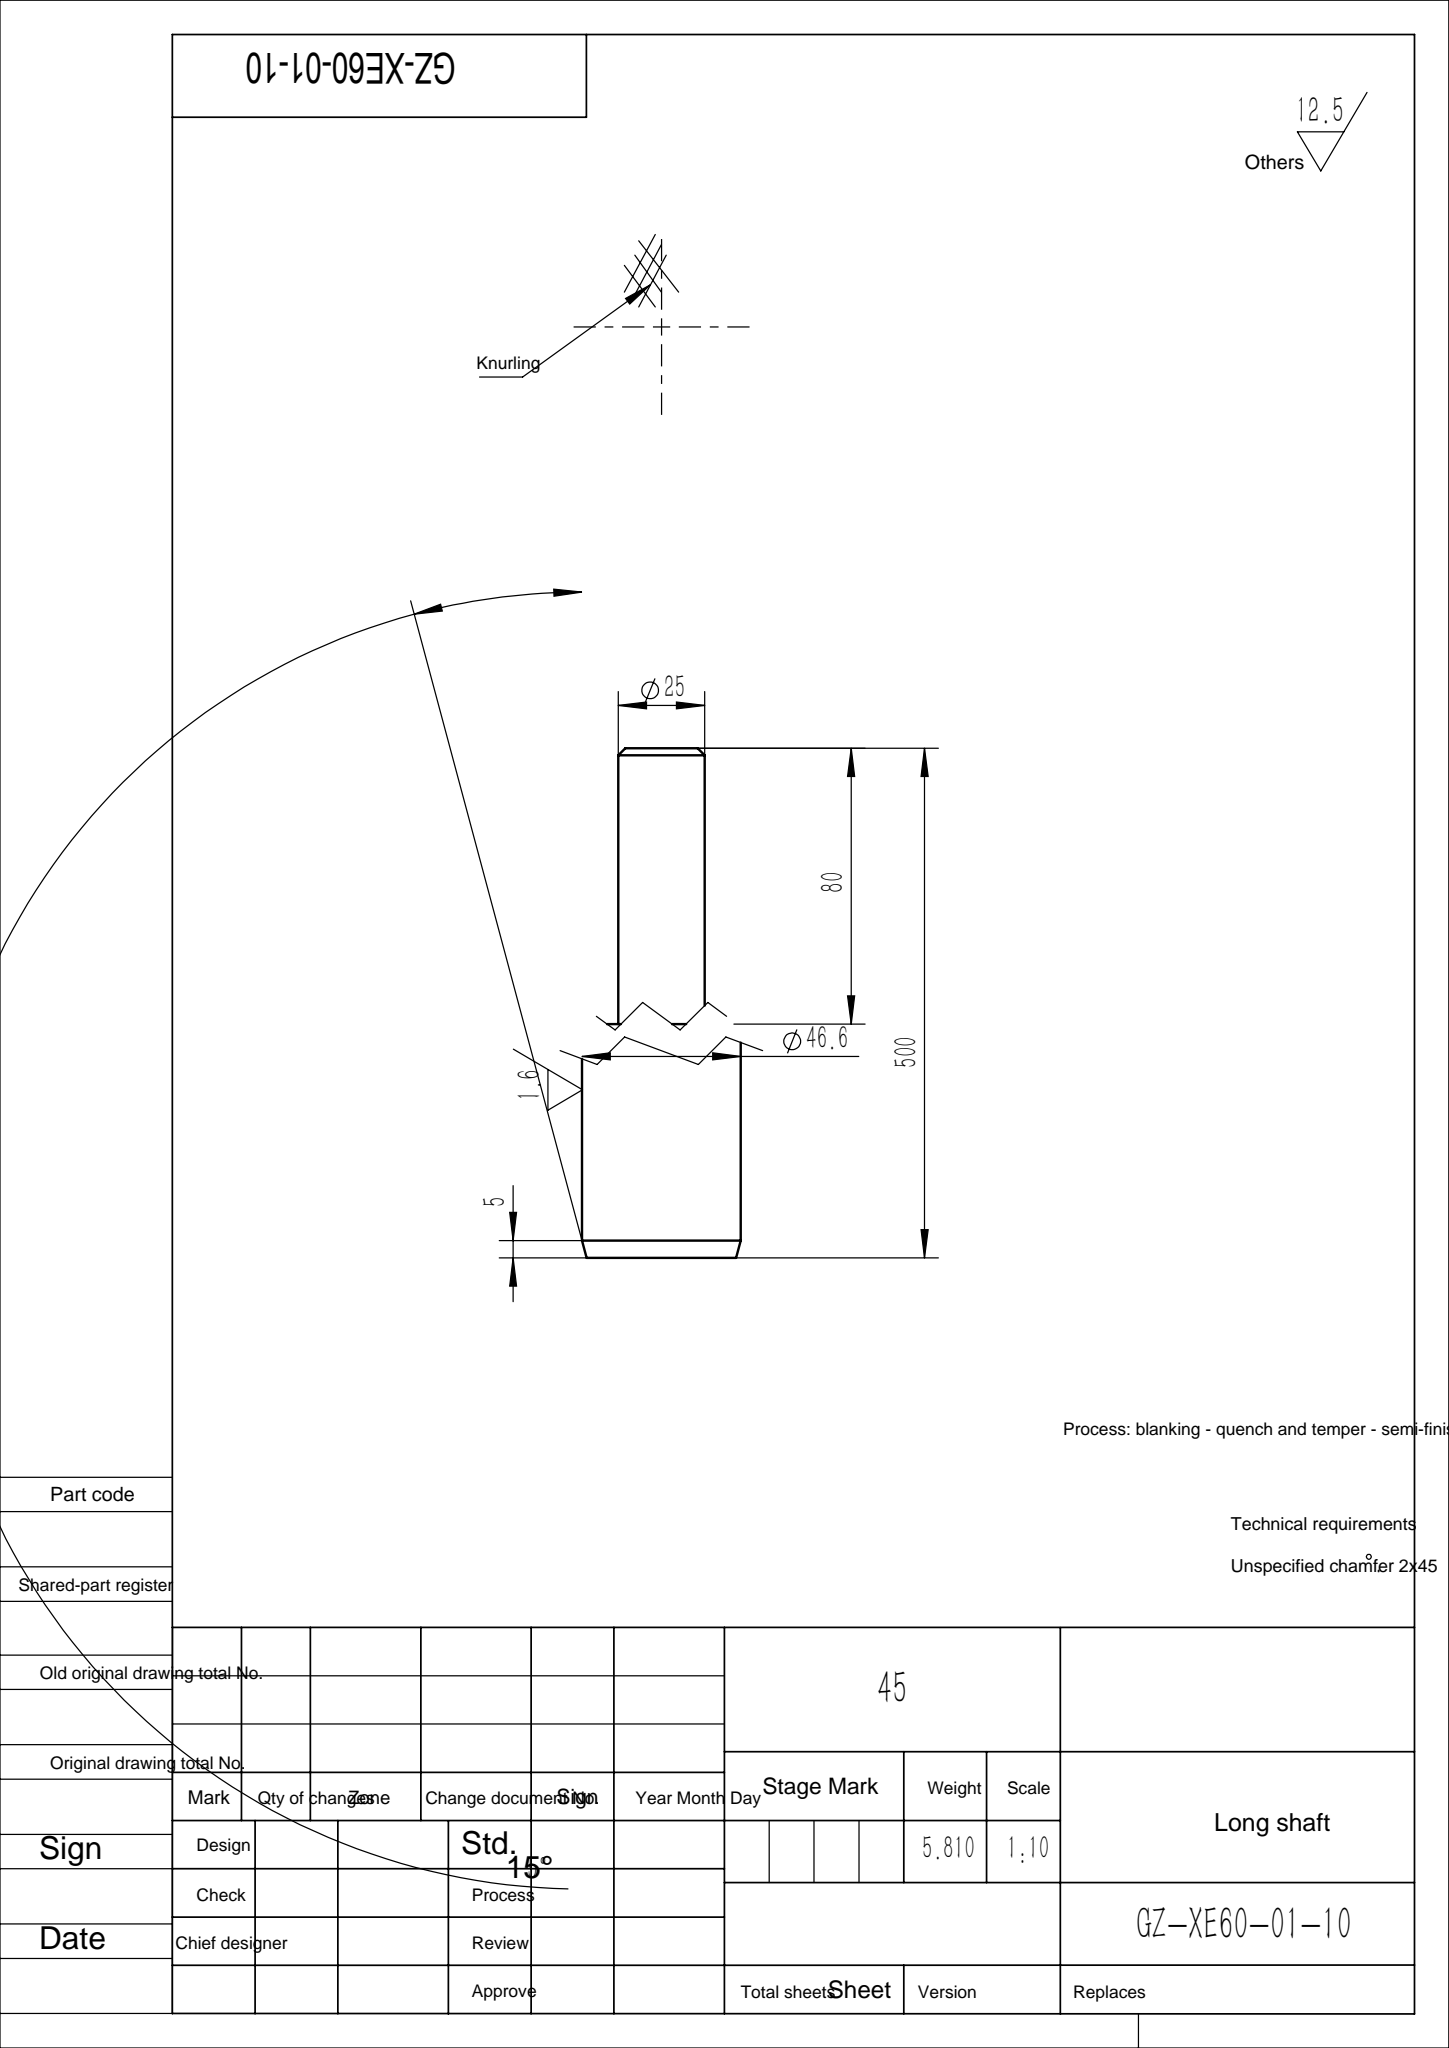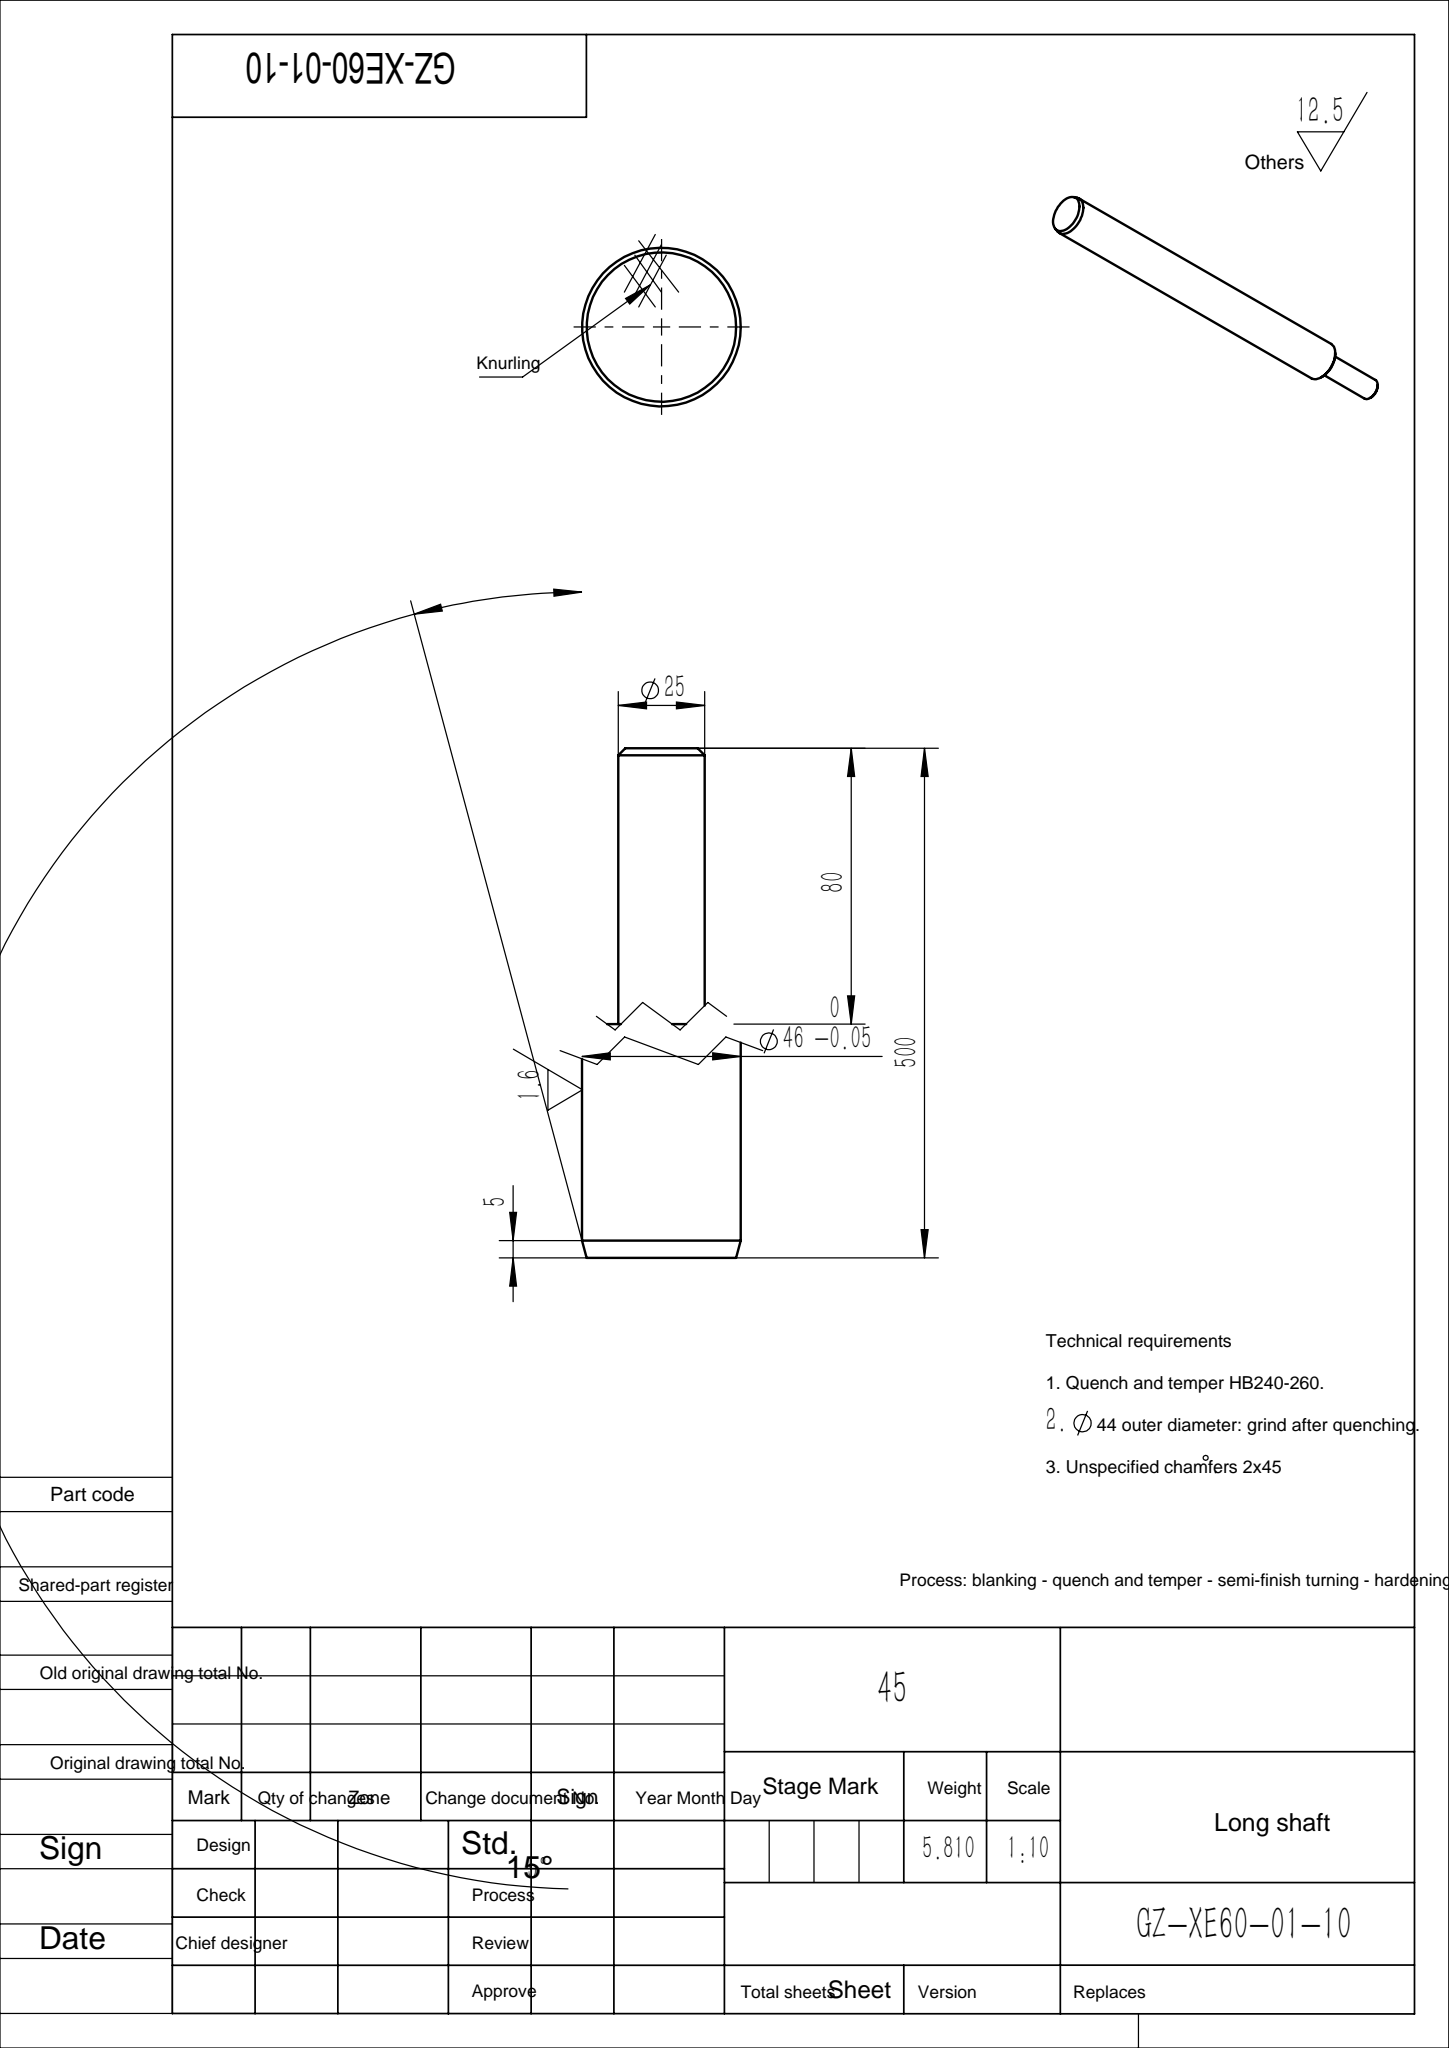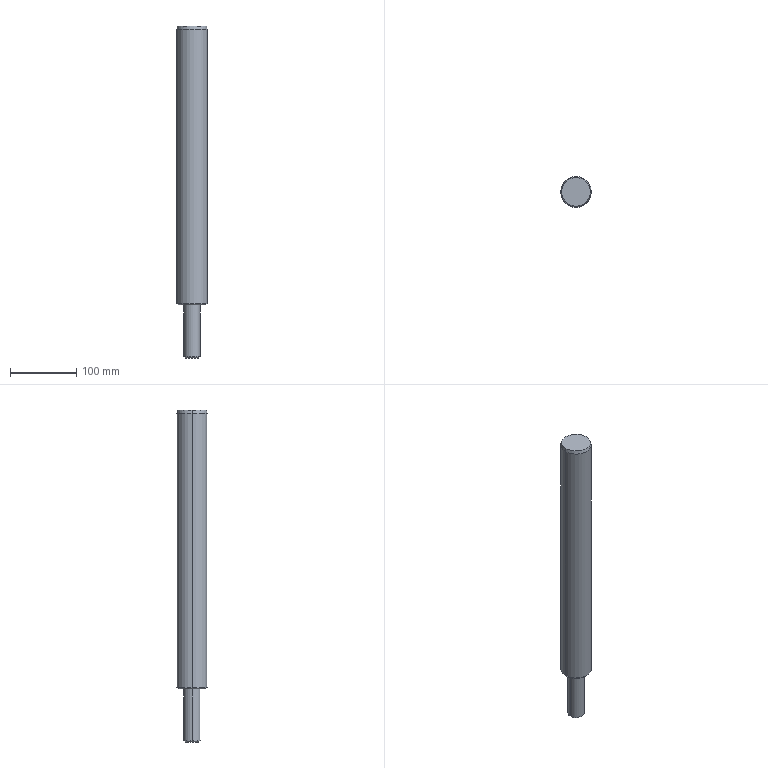Part | SolidWorks | features Chamfer 2, Extrusion 1, ICE 1 | 1 solid | 13 faces | box 46 x 46 x 500 mm | volume 736365 mm3 | cone 6 | cylinder 4 | plane 3 | commonest cylinder face diameters 25 x2 46 x2
STEP:
#1=CARTESIAN_POINT('',(-10.5,0.,-80.));
#2=VERTEX_POINT('',#1);
#3=CARTESIAN_POINT('',(10.5,0.,-80.));
#4=VERTEX_POINT('',#3);
#5=CARTESIAN_POINT('',(0.,0.,-80.));
#6=DIRECTION('',(0.,0.,-1.));
#7=DIRECTION('',(-1.,0.,0.));
#8=AXIS2_PLACEMENT_3D('',#5,#6,#7);
#9=CIRCLE('',#8,10.5);
#10=EDGE_CURVE('',#2,#4,#9,.T.);
#11=ORIENTED_EDGE('',*,*,#10,.F.);
#12=CARTESIAN_POINT('',(-12.5,0.,-78.));
#13=VERTEX_POINT('',#12);
#14=CARTESIAN_POINT('',(-10.5,0.,-80.));
#15=DIRECTION('',(-0.7071,0.,0.7071));
#16=VECTOR('',#15,1000.);
#17=LINE('',#14,#16);
#18=EDGE_CURVE('',#2,#13,#17,.T.);
#19=ORIENTED_EDGE('',*,*,#18,.T.);
#20=CARTESIAN_POINT('',(12.5,0.,-78.));
#21=VERTEX_POINT('',#20);
#22=CARTESIAN_POINT('',(0.,0.,-78.));
#23=DIRECTION('',(0.,0.,1.));
#24=DIRECTION('',(-1.,0.,0.));
#25=AXIS2_PLACEMENT_3D('',#22,#23,#24);
#26=CIRCLE('',#25,12.5);
#27=EDGE_CURVE('',#21,#13,#26,.T.);
#28=ORIENTED_EDGE('',*,*,#27,.F.);
#29=CARTESIAN_POINT('',(10.5,0.,-80.));
#30=DIRECTION('',(0.7071,0.,0.7071));
#31=VECTOR('',#30,1000.);
#32=LINE('',#29,#31);
#33=EDGE_CURVE('',#4,#21,#32,.T.);
#34=ORIENTED_EDGE('',*,*,#33,.F.);
#35=EDGE_LOOP('',(#11,#19,#28,#34));
#36=FACE_OUTER_BOUND('',#35,.T.);
#37=CARTESIAN_POINT('',(0.,0.,-80.));
#38=DIRECTION('',(0.,0.,1.));
#39=DIRECTION('',(1.,0.,0.));
#40=AXIS2_PLACEMENT_3D('',#37,#38,#39);
#41=CONICAL_SURFACE('',#40,10.5,0.7854);
#42=ADVANCED_FACE('',(#36),#41,.T.);
#43=CARTESIAN_POINT('',(-21.,0.,0.));
#44=VERTEX_POINT('',#43);
#45=CARTESIAN_POINT('',(21.,0.,0.));
#46=VERTEX_POINT('',#45);
#47=CARTESIAN_POINT('',(0.,0.,0.));
#48=DIRECTION('',(0.,0.,-1.));
#49=DIRECTION('',(1.,0.,0.));
#50=AXIS2_PLACEMENT_3D('',#47,#48,#49);
#51=CIRCLE('',#50,21.);
#52=EDGE_CURVE('',#44,#46,#51,.T.);
#53=ORIENTED_EDGE('',*,*,#52,.F.);
#54=CARTESIAN_POINT('',(-23.,0.,2.));
#55=VERTEX_POINT('',#54);
#56=CARTESIAN_POINT('',(-23.,0.,2.));
#57=DIRECTION('',(-0.7071,0.,0.7071));
#58=VECTOR('',#57,1000.);
#59=LINE('',#56,#58);
#60=EDGE_CURVE('',#44,#55,#59,.T.);
#61=ORIENTED_EDGE('',*,*,#60,.T.);
#62=CARTESIAN_POINT('',(23.,0.,2.));
#63=VERTEX_POINT('',#62);
#64=CARTESIAN_POINT('',(0.,0.,2.));
#65=DIRECTION('',(0.,0.,1.));
#66=DIRECTION('',(1.,0.,0.));
#67=AXIS2_PLACEMENT_3D('',#64,#65,#66);
#68=CIRCLE('',#67,23.);
#69=EDGE_CURVE('',#63,#55,#68,.T.);
#70=ORIENTED_EDGE('',*,*,#69,.F.);
#71=CARTESIAN_POINT('',(23.,0.,2.));
#72=DIRECTION('',(0.7071,0.,0.7071));
#73=VECTOR('',#72,1000.);
#74=LINE('',#71,#73);
#75=EDGE_CURVE('',#46,#63,#74,.T.);
#76=ORIENTED_EDGE('',*,*,#75,.F.);
#77=EDGE_LOOP('',(#53,#61,#70,#76));
#78=FACE_OUTER_BOUND('',#77,.T.);
#79=CARTESIAN_POINT('',(0.,0.,2.));
#80=DIRECTION('',(0.,0.,1.));
#81=DIRECTION('',(1.,0.,0.));
#82=AXIS2_PLACEMENT_3D('',#79,#80,#81);
#83=CONICAL_SURFACE('',#82,23.,0.7854);
#84=ADVANCED_FACE('',(#78),#83,.T.);
#85=ORIENTED_EDGE('',*,*,#27,.T.);
#86=CARTESIAN_POINT('',(-12.5,0.,0.));
#87=VERTEX_POINT('',#86);
#88=CARTESIAN_POINT('',(-12.5,0.,-80.));
#89=DIRECTION('',(0.,0.,1.));
#90=VECTOR('',#89,1000.);
#91=LINE('',#88,#90);
#92=EDGE_CURVE('',#13,#87,#91,.T.);
#93=ORIENTED_EDGE('',*,*,#92,.T.);
#94=CARTESIAN_POINT('',(12.5,0.,0.));
#95=VERTEX_POINT('',#94);
#96=CARTESIAN_POINT('',(0.,0.,0.));
#97=DIRECTION('',(0.,0.,-1.));
#98=DIRECTION('',(1.,0.,0.));
#99=AXIS2_PLACEMENT_3D('',#96,#97,#98);
#100=CIRCLE('',#99,12.5);
#101=EDGE_CURVE('',#87,#95,#100,.T.);
#102=ORIENTED_EDGE('',*,*,#101,.T.);
#103=CARTESIAN_POINT('',(12.5,0.,-80.));
#104=DIRECTION('',(0.,0.,1.));
#105=VECTOR('',#104,1000.);
#106=LINE('',#103,#105);
#107=EDGE_CURVE('',#21,#95,#106,.T.);
#108=ORIENTED_EDGE('',*,*,#107,.F.);
#109=EDGE_LOOP('',(#85,#93,#102,#108));
#110=FACE_OUTER_BOUND('',#109,.T.);
#111=CARTESIAN_POINT('',(0.,0.,-80.));
#112=DIRECTION('',(0.,0.,1.));
#113=DIRECTION('',(1.,0.,0.));
#114=AXIS2_PLACEMENT_3D('',#111,#112,#113);
#115=CYLINDRICAL_SURFACE('',#114,12.5);
#116=ADVANCED_FACE('',(#110),#115,.T.);
#117=CARTESIAN_POINT('',(21.66,0.,420.));
#118=VERTEX_POINT('',#117);
#119=CARTESIAN_POINT('',(-21.66,0.,420.));
#120=VERTEX_POINT('',#119);
#121=CARTESIAN_POINT('',(0.,0.,420.));
#122=DIRECTION('',(0.,0.,1.));
#123=DIRECTION('',(1.,0.,0.));
#124=AXIS2_PLACEMENT_3D('',#121,#122,#123);
#125=CIRCLE('',#124,21.66);
#126=EDGE_CURVE('',#118,#120,#125,.T.);
#127=ORIENTED_EDGE('',*,*,#126,.F.);
#128=CARTESIAN_POINT('',(23.,0.,415.));
#129=VERTEX_POINT('',#128);
#130=CARTESIAN_POINT('',(21.66,0.,420.));
#131=DIRECTION('',(0.2588,0.,-0.9659));
#132=VECTOR('',#131,1000.);
#133=LINE('',#130,#132);
#134=EDGE_CURVE('',#118,#129,#133,.T.);
#135=ORIENTED_EDGE('',*,*,#134,.T.);
#136=CARTESIAN_POINT('',(-23.,0.,415.));
#137=VERTEX_POINT('',#136);
#138=CARTESIAN_POINT('',(0.,0.,415.));
#139=DIRECTION('',(0.,0.,-1.));
#140=DIRECTION('',(1.,0.,0.));
#141=AXIS2_PLACEMENT_3D('',#138,#139,#140);
#142=CIRCLE('',#141,23.);
#143=EDGE_CURVE('',#137,#129,#142,.T.);
#144=ORIENTED_EDGE('',*,*,#143,.F.);
#145=CARTESIAN_POINT('',(-21.66,0.,420.));
#146=DIRECTION('',(-0.2588,0.,-0.9659));
#147=VECTOR('',#146,1000.);
#148=LINE('',#145,#147);
#149=EDGE_CURVE('',#120,#137,#148,.T.);
#150=ORIENTED_EDGE('',*,*,#149,.F.);
#151=EDGE_LOOP('',(#127,#135,#144,#150));
#152=FACE_OUTER_BOUND('',#151,.T.);
#153=CARTESIAN_POINT('',(0.,0.,420.));
#154=DIRECTION('',(0.,0.,-1.));
#155=DIRECTION('',(-1.,0.,0.));
#156=AXIS2_PLACEMENT_3D('',#153,#154,#155);
#157=CONICAL_SURFACE('',#156,21.66,0.2618);
#158=ADVANCED_FACE('',(#152),#157,.T.);
#159=ORIENTED_EDGE('',*,*,#143,.T.);
#160=CARTESIAN_POINT('',(23.,0.,420.));
#161=DIRECTION('',(0.,0.,-1.));
#162=VECTOR('',#161,1000.);
#163=LINE('',#160,#162);
#164=EDGE_CURVE('',#129,#63,#163,.T.);
#165=ORIENTED_EDGE('',*,*,#164,.T.);
#166=ORIENTED_EDGE('',*,*,#69,.T.);
#167=CARTESIAN_POINT('',(-23.,0.,420.));
#168=DIRECTION('',(0.,0.,-1.));
#169=VECTOR('',#168,1000.);
#170=LINE('',#167,#169);
#171=EDGE_CURVE('',#137,#55,#170,.T.);
#172=ORIENTED_EDGE('',*,*,#171,.F.);
#173=EDGE_LOOP('',(#159,#165,#166,#172));
#174=FACE_OUTER_BOUND('',#173,.T.);
#175=CARTESIAN_POINT('',(0.,0.,420.));
#176=DIRECTION('',(0.,0.,-1.));
#177=DIRECTION('',(-1.,0.,0.));
#178=AXIS2_PLACEMENT_3D('',#175,#176,#177);
#179=CYLINDRICAL_SURFACE('',#178,23.);
#180=ADVANCED_FACE('',(#174),#179,.T.);
#181=ORIENTED_EDGE('',*,*,#164,.F.);
#182=CARTESIAN_POINT('',(0.,0.,415.));
#183=DIRECTION('',(0.,0.,-1.));
#184=DIRECTION('',(1.,0.,0.));
#185=AXIS2_PLACEMENT_3D('',#182,#183,#184);
#186=CIRCLE('',#185,23.);
#187=EDGE_CURVE('',#129,#137,#186,.T.);
#188=ORIENTED_EDGE('',*,*,#187,.T.);
#189=ORIENTED_EDGE('',*,*,#171,.T.);
#190=CARTESIAN_POINT('',(0.,0.,2.));
#191=DIRECTION('',(0.,0.,1.));
#192=DIRECTION('',(1.,0.,0.));
#193=AXIS2_PLACEMENT_3D('',#190,#191,#192);
#194=CIRCLE('',#193,23.);
#195=EDGE_CURVE('',#55,#63,#194,.T.);
#196=ORIENTED_EDGE('',*,*,#195,.T.);
#197=EDGE_LOOP('',(#181,#188,#189,#196));
#198=FACE_OUTER_BOUND('',#197,.T.);
#199=CARTESIAN_POINT('',(0.,0.,420.));
#200=DIRECTION('',(0.,0.,-1.));
#201=DIRECTION('',(-1.,0.,0.));
#202=AXIS2_PLACEMENT_3D('',#199,#200,#201);
#203=CYLINDRICAL_SURFACE('',#202,23.);
#204=ADVANCED_FACE('',(#198),#203,.T.);
#205=CARTESIAN_POINT('',(0.,0.,420.));
#206=DIRECTION('',(0.,0.,1.));
#207=DIRECTION('',(1.,0.,0.));
#208=AXIS2_PLACEMENT_3D('',#205,#206,#207);
#209=CIRCLE('',#208,21.66);
#210=EDGE_CURVE('',#120,#118,#209,.T.);
#211=ORIENTED_EDGE('',*,*,#210,.T.);
#212=ORIENTED_EDGE('',*,*,#126,.T.);
#213=EDGE_LOOP('',(#211,#212));
#214=FACE_OUTER_BOUND('',#213,.T.);
#215=CARTESIAN_POINT('',(0.,0.,420.));
#216=DIRECTION('',(0.,0.,1.));
#217=DIRECTION('',(1.,0.,0.));
#218=AXIS2_PLACEMENT_3D('',#215,#216,#217);
#219=PLANE('',#218);
#220=ADVANCED_FACE('',(#214),#219,.T.);
#221=CARTESIAN_POINT('',(0.,0.,0.));
#222=DIRECTION('',(0.,0.,-1.));
#223=DIRECTION('',(1.,0.,0.));
#224=AXIS2_PLACEMENT_3D('',#221,#222,#223);
#225=CIRCLE('',#224,21.);
#226=EDGE_CURVE('',#46,#44,#225,.T.);
#227=ORIENTED_EDGE('',*,*,#226,.T.);
#228=ORIENTED_EDGE('',*,*,#52,.T.);
#229=EDGE_LOOP('',(#227,#228));
#230=FACE_OUTER_BOUND('',#229,.T.);
#231=CARTESIAN_POINT('',(0.,0.,0.));
#232=DIRECTION('',(0.,0.,-1.));
#233=DIRECTION('',(1.,0.,0.));
#234=AXIS2_PLACEMENT_3D('',#231,#232,#233);
#235=CIRCLE('',#234,12.5);
#236=EDGE_CURVE('',#95,#87,#235,.T.);
#237=ORIENTED_EDGE('',*,*,#236,.F.);
#238=ORIENTED_EDGE('',*,*,#101,.F.);
#239=EDGE_LOOP('',(#237,#238));
#240=FACE_BOUND('',#239,.T.);
#241=CARTESIAN_POINT('',(0.,0.,0.));
#242=DIRECTION('',(0.,0.,1.));
#243=DIRECTION('',(1.,0.,0.));
#244=AXIS2_PLACEMENT_3D('',#241,#242,#243);
#245=PLANE('',#244);
#246=ADVANCED_FACE('',(#230,#240),#245,.F.);
#247=ORIENTED_EDGE('',*,*,#134,.F.);
#248=ORIENTED_EDGE('',*,*,#210,.F.);
#249=ORIENTED_EDGE('',*,*,#149,.T.);
#250=ORIENTED_EDGE('',*,*,#187,.F.);
#251=EDGE_LOOP('',(#247,#248,#249,#250));
#252=FACE_OUTER_BOUND('',#251,.T.);
#253=CARTESIAN_POINT('',(0.,0.,420.));
#254=DIRECTION('',(0.,0.,-1.));
#255=DIRECTION('',(-1.,0.,0.));
#256=AXIS2_PLACEMENT_3D('',#253,#254,#255);
#257=CONICAL_SURFACE('',#256,21.66,0.2618);
#258=ADVANCED_FACE('',(#252),#257,.T.);
#259=ORIENTED_EDGE('',*,*,#92,.F.);
#260=CARTESIAN_POINT('',(0.,0.,-78.));
#261=DIRECTION('',(0.,0.,1.));
#262=DIRECTION('',(-1.,0.,0.));
#263=AXIS2_PLACEMENT_3D('',#260,#261,#262);
#264=CIRCLE('',#263,12.5);
#265=EDGE_CURVE('',#13,#21,#264,.T.);
#266=ORIENTED_EDGE('',*,*,#265,.T.);
#267=ORIENTED_EDGE('',*,*,#107,.T.);
#268=ORIENTED_EDGE('',*,*,#236,.T.);
#269=EDGE_LOOP('',(#259,#266,#267,#268));
#270=FACE_OUTER_BOUND('',#269,.T.);
#271=CARTESIAN_POINT('',(0.,0.,-80.));
#272=DIRECTION('',(0.,0.,1.));
#273=DIRECTION('',(1.,0.,0.));
#274=AXIS2_PLACEMENT_3D('',#271,#272,#273);
#275=CYLINDRICAL_SURFACE('',#274,12.5);
#276=ADVANCED_FACE('',(#270),#275,.T.);
#277=CARTESIAN_POINT('',(0.,0.,-80.));
#278=DIRECTION('',(0.,0.,-1.));
#279=DIRECTION('',(-1.,0.,0.));
#280=AXIS2_PLACEMENT_3D('',#277,#278,#279);
#281=CIRCLE('',#280,10.5);
#282=EDGE_CURVE('',#4,#2,#281,.T.);
#283=ORIENTED_EDGE('',*,*,#282,.T.);
#284=ORIENTED_EDGE('',*,*,#10,.T.);
#285=EDGE_LOOP('',(#283,#284));
#286=FACE_OUTER_BOUND('',#285,.T.);
#287=CARTESIAN_POINT('',(0.,0.,-80.));
#288=DIRECTION('',(0.,0.,-1.));
#289=DIRECTION('',(-1.,0.,0.));
#290=AXIS2_PLACEMENT_3D('',#287,#288,#289);
#291=PLANE('',#290);
#292=ADVANCED_FACE('',(#286),#291,.T.);
#293=ORIENTED_EDGE('',*,*,#60,.F.);
#294=ORIENTED_EDGE('',*,*,#226,.F.);
#295=ORIENTED_EDGE('',*,*,#75,.T.);
#296=ORIENTED_EDGE('',*,*,#195,.F.);
#297=EDGE_LOOP('',(#293,#294,#295,#296));
#298=FACE_OUTER_BOUND('',#297,.T.);
#299=CARTESIAN_POINT('',(0.,0.,2.));
#300=DIRECTION('',(0.,0.,1.));
#301=DIRECTION('',(1.,0.,0.));
#302=AXIS2_PLACEMENT_3D('',#299,#300,#301);
#303=CONICAL_SURFACE('',#302,23.,0.7854);
#304=ADVANCED_FACE('',(#298),#303,.T.);
#305=ORIENTED_EDGE('',*,*,#18,.F.);
#306=ORIENTED_EDGE('',*,*,#282,.F.);
#307=ORIENTED_EDGE('',*,*,#33,.T.);
#308=ORIENTED_EDGE('',*,*,#265,.F.);
#309=EDGE_LOOP('',(#305,#306,#307,#308));
#310=FACE_OUTER_BOUND('',#309,.T.);
#311=CARTESIAN_POINT('',(0.,0.,-80.));
#312=DIRECTION('',(0.,0.,1.));
#313=DIRECTION('',(1.,0.,0.));
#314=AXIS2_PLACEMENT_3D('',#311,#312,#313);
#315=CONICAL_SURFACE('',#314,10.5,0.7854);
#316=ADVANCED_FACE('',(#310),#315,.T.);
#317=CLOSED_SHELL('',(#42,#84,#116,#158,#180,#204,#220,#246,#258,#276,#292,#304,#316));
#318=MANIFOLD_SOLID_BREP('',#317);
#319=CARTESIAN_POINT('',(0.,0.,0.));
#320=DIRECTION('',(0.,0.,1.));
#321=DIRECTION('',(1.,0.,0.));
#322=AXIS2_PLACEMENT_3D('',#319,#320,#321);
#323=(LENGTH_UNIT()NAMED_UNIT(*)SI_UNIT(.MILLI.,.METRE.));
#324=UNCERTAINTY_MEASURE_WITH_UNIT(LENGTH_MEASURE(0.00001),#323,'','');
#325=(NAMED_UNIT(*)PLANE_ANGLE_UNIT()SI_UNIT($,.RADIAN.));
#326=(NAMED_UNIT(*)SI_UNIT($,.STERADIAN.)SOLID_ANGLE_UNIT());
#327=(GEOMETRIC_REPRESENTATION_CONTEXT(3)GLOBAL_UNCERTAINTY_ASSIGNED_CONTEXT((#324))GLOBAL_UNIT_ASSIGNED_CONTEXT((#323,#325,#326))REPRESENTATION_CONTEXT('',''));
#328=ADVANCED_BREP_SHAPE_REPRESENTATION('',(#318,#322),#327);